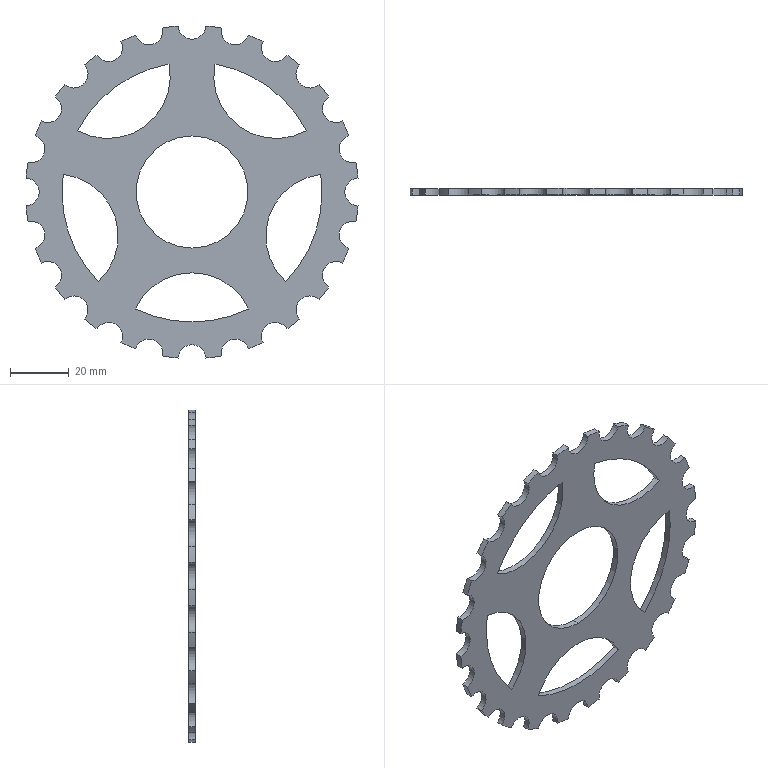Part | STEP file | Gear | 1 solid | 74 faces | box 113.111 x 2.2 x 113.111 mm | volume 12913 mm3 | cylinder 72 | plane 2 | commonest cylinder face diameters 9.4 x35 113.5 x24 42.486 x6 88.569 x5 38.2 x2